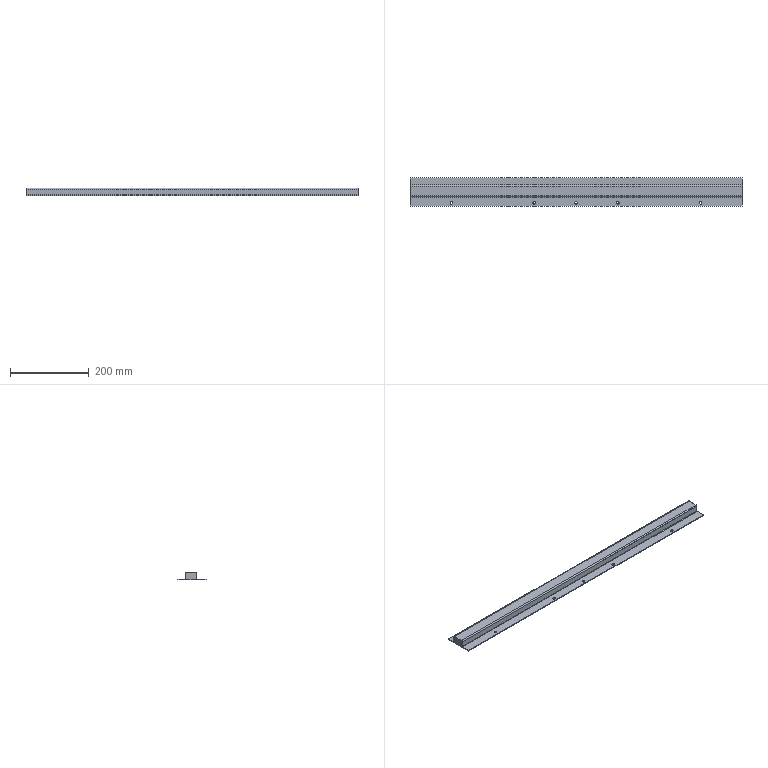Part | SolidWorks | features BaseBody 3 | 3 solids | 64 faces | box 841.8 x 71 x 20 mm | volume 175903 mm3 | plane 42 | cylinder 22 | commonest cylinder face diameters 6.5 x10 2 x8 6 x4